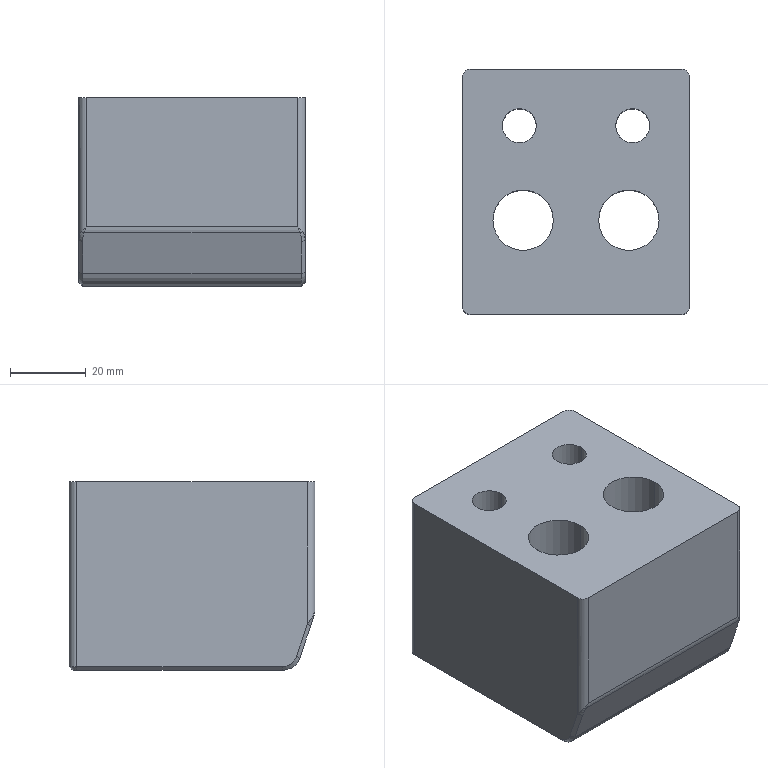Part | SolidWorks | features BaseBody 1 | 1 solid | 97 faces | box 60 x 65 x 50 mm | volume 160971 mm3 | cylinder 58 | plane 21 | cone 14 | spline 4 | commonest cylinder face diameters 2 x12 6 x12 2.5 x8 4 x4 9 x4 15 x4